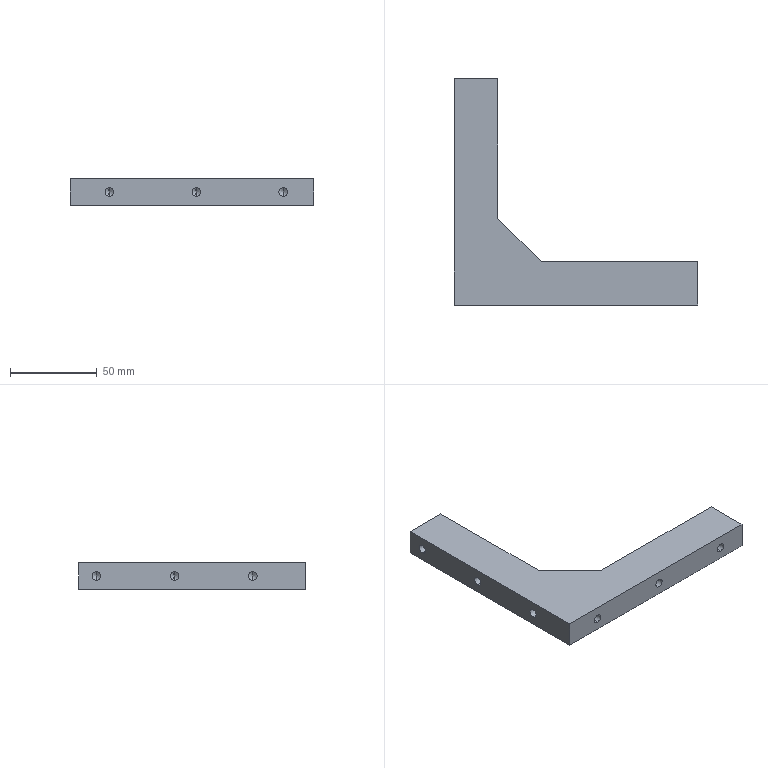Part | SolidWorks | features 3DProfileFeature 1, Extrusion 1, HoleWzd 1 | 1 solid | 33 faces | box 140 x 130 x 15 mm | volume 95031 mm3 | cylinder 12 | cone 12 | plane 9 | commonest cylinder face diameters 5 x12
STEP:
#1=CARTESIAN_POINT('',(122.5,12.5,2.5));
#2=VERTEX_POINT('',#1);
#3=CARTESIAN_POINT('',(122.5,12.5,-2.5));
#4=VERTEX_POINT('',#3);
#5=CARTESIAN_POINT('',(122.5,12.5,0.));
#6=DIRECTION('',(0.,-1.,0.));
#7=DIRECTION('',(0.,0.,-1.));
#8=AXIS2_PLACEMENT_3D('',#5,#6,#7);
#9=CIRCLE('',#8,2.5);
#10=EDGE_CURVE('',#2,#4,#9,.T.);
#11=ORIENTED_EDGE('',*,*,#10,.F.);
#12=CARTESIAN_POINT('',(122.5,0.,2.5));
#13=VERTEX_POINT('',#12);
#14=CARTESIAN_POINT('',(122.5,0.,2.5));
#15=DIRECTION('',(0.,-1.,0.));
#16=VECTOR('',#15,1000.);
#17=LINE('',#14,#16);
#18=EDGE_CURVE('',#2,#13,#17,.T.);
#19=ORIENTED_EDGE('',*,*,#18,.T.);
#20=CARTESIAN_POINT('',(122.5,0.,-2.5));
#21=VERTEX_POINT('',#20);
#22=CARTESIAN_POINT('',(122.5,0.,0.));
#23=DIRECTION('',(0.,-1.,0.));
#24=DIRECTION('',(0.,0.,-1.));
#25=AXIS2_PLACEMENT_3D('',#22,#23,#24);
#26=CIRCLE('',#25,2.5);
#27=EDGE_CURVE('',#13,#21,#26,.T.);
#28=ORIENTED_EDGE('',*,*,#27,.T.);
#29=CARTESIAN_POINT('',(122.5,0.,-2.5));
#30=DIRECTION('',(0.,-1.,0.));
#31=VECTOR('',#30,1000.);
#32=LINE('',#29,#31);
#33=EDGE_CURVE('',#4,#21,#32,.T.);
#34=ORIENTED_EDGE('',*,*,#33,.F.);
#35=EDGE_LOOP('',(#11,#19,#28,#34));
#36=FACE_OUTER_BOUND('',#35,.T.);
#37=CARTESIAN_POINT('',(122.5,0.,0.));
#38=DIRECTION('',(0.,-1.,0.));
#39=DIRECTION('',(0.,0.,-1.));
#40=AXIS2_PLACEMENT_3D('',#37,#38,#39);
#41=CYLINDRICAL_SURFACE('',#40,2.5);
#42=ADVANCED_FACE('',(#36),#41,.F.);
#43=CARTESIAN_POINT('',(122.5,14.002,0.));
#44=VERTEX_POINT('',#43);
#45=CARTESIAN_POINT('',(122.5,12.5,-2.5));
#46=DIRECTION('',(0.,-0.515,-0.8572));
#47=VECTOR('',#46,1000.);
#48=LINE('',#45,#47);
#49=EDGE_CURVE('',#44,#4,#48,.T.);
#50=ORIENTED_EDGE('',*,*,#49,.F.);
#51=CARTESIAN_POINT('',(122.5,12.5,2.5));
#52=DIRECTION('',(0.,-0.515,0.8572));
#53=VECTOR('',#52,1000.);
#54=LINE('',#51,#53);
#55=EDGE_CURVE('',#44,#2,#54,.T.);
#56=ORIENTED_EDGE('',*,*,#55,.T.);
#57=ORIENTED_EDGE('',*,*,#10,.T.);
#58=EDGE_LOOP('',(#50,#56,#57));
#59=FACE_OUTER_BOUND('',#58,.T.);
#60=CARTESIAN_POINT('',(122.5,12.5,0.));
#61=DIRECTION('',(0.,-1.,0.));
#62=DIRECTION('',(0.,0.,-1.));
#63=AXIS2_PLACEMENT_3D('',#60,#61,#62);
#64=CONICAL_SURFACE('',#63,2.5,1.03);
#65=ADVANCED_FACE('',(#59),#64,.F.);
#66=CARTESIAN_POINT('',(72.5,12.5,2.5));
#67=VERTEX_POINT('',#66);
#68=CARTESIAN_POINT('',(72.5,12.5,-2.5));
#69=VERTEX_POINT('',#68);
#70=CARTESIAN_POINT('',(72.5,12.5,0.));
#71=DIRECTION('',(0.,-1.,0.));
#72=DIRECTION('',(0.,0.,-1.));
#73=AXIS2_PLACEMENT_3D('',#70,#71,#72);
#74=CIRCLE('',#73,2.5);
#75=EDGE_CURVE('',#67,#69,#74,.T.);
#76=ORIENTED_EDGE('',*,*,#75,.F.);
#77=CARTESIAN_POINT('',(72.5,0.,2.5));
#78=VERTEX_POINT('',#77);
#79=CARTESIAN_POINT('',(72.5,0.,2.5));
#80=DIRECTION('',(0.,-1.,0.));
#81=VECTOR('',#80,1000.);
#82=LINE('',#79,#81);
#83=EDGE_CURVE('',#67,#78,#82,.T.);
#84=ORIENTED_EDGE('',*,*,#83,.T.);
#85=CARTESIAN_POINT('',(72.5,0.,-2.5));
#86=VERTEX_POINT('',#85);
#87=CARTESIAN_POINT('',(72.5,0.,0.));
#88=DIRECTION('',(0.,-1.,0.));
#89=DIRECTION('',(0.,0.,-1.));
#90=AXIS2_PLACEMENT_3D('',#87,#88,#89);
#91=CIRCLE('',#90,2.5);
#92=EDGE_CURVE('',#78,#86,#91,.T.);
#93=ORIENTED_EDGE('',*,*,#92,.T.);
#94=CARTESIAN_POINT('',(72.5,0.,-2.5));
#95=DIRECTION('',(0.,-1.,0.));
#96=VECTOR('',#95,1000.);
#97=LINE('',#94,#96);
#98=EDGE_CURVE('',#69,#86,#97,.T.);
#99=ORIENTED_EDGE('',*,*,#98,.F.);
#100=EDGE_LOOP('',(#76,#84,#93,#99));
#101=FACE_OUTER_BOUND('',#100,.T.);
#102=CARTESIAN_POINT('',(72.5,0.,0.));
#103=DIRECTION('',(0.,-1.,0.));
#104=DIRECTION('',(0.,0.,-1.));
#105=AXIS2_PLACEMENT_3D('',#102,#103,#104);
#106=CYLINDRICAL_SURFACE('',#105,2.5);
#107=ADVANCED_FACE('',(#101),#106,.F.);
#108=CARTESIAN_POINT('',(72.5,14.002,0.));
#109=VERTEX_POINT('',#108);
#110=CARTESIAN_POINT('',(72.5,12.5,-2.5));
#111=DIRECTION('',(0.,-0.515,-0.8572));
#112=VECTOR('',#111,1000.);
#113=LINE('',#110,#112);
#114=EDGE_CURVE('',#109,#69,#113,.T.);
#115=ORIENTED_EDGE('',*,*,#114,.F.);
#116=CARTESIAN_POINT('',(72.5,12.5,2.5));
#117=DIRECTION('',(0.,-0.515,0.8572));
#118=VECTOR('',#117,1000.);
#119=LINE('',#116,#118);
#120=EDGE_CURVE('',#109,#67,#119,.T.);
#121=ORIENTED_EDGE('',*,*,#120,.T.);
#122=ORIENTED_EDGE('',*,*,#75,.T.);
#123=EDGE_LOOP('',(#115,#121,#122));
#124=FACE_OUTER_BOUND('',#123,.T.);
#125=CARTESIAN_POINT('',(72.5,12.5,0.));
#126=DIRECTION('',(0.,-1.,0.));
#127=DIRECTION('',(0.,0.,-1.));
#128=AXIS2_PLACEMENT_3D('',#125,#126,#127);
#129=CONICAL_SURFACE('',#128,2.5,1.03);
#130=ADVANCED_FACE('',(#124),#129,.F.);
#131=CARTESIAN_POINT('',(22.5,12.5,2.5));
#132=VERTEX_POINT('',#131);
#133=CARTESIAN_POINT('',(22.5,12.5,-2.5));
#134=VERTEX_POINT('',#133);
#135=CARTESIAN_POINT('',(22.5,12.5,0.));
#136=DIRECTION('',(0.,-1.,0.));
#137=DIRECTION('',(0.,0.,-1.));
#138=AXIS2_PLACEMENT_3D('',#135,#136,#137);
#139=CIRCLE('',#138,2.5);
#140=EDGE_CURVE('',#132,#134,#139,.T.);
#141=ORIENTED_EDGE('',*,*,#140,.F.);
#142=CARTESIAN_POINT('',(22.5,0.,2.5));
#143=VERTEX_POINT('',#142);
#144=CARTESIAN_POINT('',(22.5,0.,2.5));
#145=DIRECTION('',(0.,-1.,0.));
#146=VECTOR('',#145,1000.);
#147=LINE('',#144,#146);
#148=EDGE_CURVE('',#132,#143,#147,.T.);
#149=ORIENTED_EDGE('',*,*,#148,.T.);
#150=CARTESIAN_POINT('',(22.5,0.,-2.5));
#151=VERTEX_POINT('',#150);
#152=CARTESIAN_POINT('',(22.5,0.,0.));
#153=DIRECTION('',(0.,-1.,0.));
#154=DIRECTION('',(0.,0.,-1.));
#155=AXIS2_PLACEMENT_3D('',#152,#153,#154);
#156=CIRCLE('',#155,2.5);
#157=EDGE_CURVE('',#143,#151,#156,.T.);
#158=ORIENTED_EDGE('',*,*,#157,.T.);
#159=CARTESIAN_POINT('',(22.5,0.,-2.5));
#160=DIRECTION('',(0.,-1.,0.));
#161=VECTOR('',#160,1000.);
#162=LINE('',#159,#161);
#163=EDGE_CURVE('',#134,#151,#162,.T.);
#164=ORIENTED_EDGE('',*,*,#163,.F.);
#165=EDGE_LOOP('',(#141,#149,#158,#164));
#166=FACE_OUTER_BOUND('',#165,.T.);
#167=CARTESIAN_POINT('',(22.5,0.,0.));
#168=DIRECTION('',(0.,-1.,0.));
#169=DIRECTION('',(0.,0.,-1.));
#170=AXIS2_PLACEMENT_3D('',#167,#168,#169);
#171=CYLINDRICAL_SURFACE('',#170,2.5);
#172=ADVANCED_FACE('',(#166),#171,.F.);
#173=CARTESIAN_POINT('',(22.5,14.002,0.));
#174=VERTEX_POINT('',#173);
#175=CARTESIAN_POINT('',(22.5,12.5,-2.5));
#176=DIRECTION('',(0.,-0.515,-0.8572));
#177=VECTOR('',#176,1000.);
#178=LINE('',#175,#177);
#179=EDGE_CURVE('',#174,#134,#178,.T.);
#180=ORIENTED_EDGE('',*,*,#179,.F.);
#181=CARTESIAN_POINT('',(22.5,12.5,2.5));
#182=DIRECTION('',(0.,-0.515,0.8572));
#183=VECTOR('',#182,1000.);
#184=LINE('',#181,#183);
#185=EDGE_CURVE('',#174,#132,#184,.T.);
#186=ORIENTED_EDGE('',*,*,#185,.T.);
#187=ORIENTED_EDGE('',*,*,#140,.T.);
#188=EDGE_LOOP('',(#180,#186,#187));
#189=FACE_OUTER_BOUND('',#188,.T.);
#190=CARTESIAN_POINT('',(22.5,12.5,0.));
#191=DIRECTION('',(0.,-1.,0.));
#192=DIRECTION('',(0.,0.,-1.));
#193=AXIS2_PLACEMENT_3D('',#190,#191,#192);
#194=CONICAL_SURFACE('',#193,2.5,1.03);
#195=ADVANCED_FACE('',(#189),#194,.F.);
#196=CARTESIAN_POINT('',(12.5,30.,-2.5));
#197=VERTEX_POINT('',#196);
#198=CARTESIAN_POINT('',(12.5,30.,2.5));
#199=VERTEX_POINT('',#198);
#200=CARTESIAN_POINT('',(12.5,30.,0.));
#201=DIRECTION('',(-1.,0.,0.));
#202=DIRECTION('',(0.,0.,1.));
#203=AXIS2_PLACEMENT_3D('',#200,#201,#202);
#204=CIRCLE('',#203,2.5);
#205=EDGE_CURVE('',#197,#199,#204,.T.);
#206=ORIENTED_EDGE('',*,*,#205,.F.);
#207=CARTESIAN_POINT('',(0.,30.,-2.5));
#208=VERTEX_POINT('',#207);
#209=CARTESIAN_POINT('',(0.,30.,-2.5));
#210=DIRECTION('',(-1.,0.,0.));
#211=VECTOR('',#210,1000.);
#212=LINE('',#209,#211);
#213=EDGE_CURVE('',#197,#208,#212,.T.);
#214=ORIENTED_EDGE('',*,*,#213,.T.);
#215=CARTESIAN_POINT('',(0.,30.,2.5));
#216=VERTEX_POINT('',#215);
#217=CARTESIAN_POINT('',(0.,30.,0.));
#218=DIRECTION('',(-1.,0.,0.));
#219=DIRECTION('',(0.,0.,1.));
#220=AXIS2_PLACEMENT_3D('',#217,#218,#219);
#221=CIRCLE('',#220,2.5);
#222=EDGE_CURVE('',#208,#216,#221,.T.);
#223=ORIENTED_EDGE('',*,*,#222,.T.);
#224=CARTESIAN_POINT('',(0.,30.,2.5));
#225=DIRECTION('',(-1.,0.,0.));
#226=VECTOR('',#225,1000.);
#227=LINE('',#224,#226);
#228=EDGE_CURVE('',#199,#216,#227,.T.);
#229=ORIENTED_EDGE('',*,*,#228,.F.);
#230=EDGE_LOOP('',(#206,#214,#223,#229));
#231=FACE_OUTER_BOUND('',#230,.T.);
#232=CARTESIAN_POINT('',(0.,30.,0.));
#233=DIRECTION('',(-1.,0.,0.));
#234=DIRECTION('',(0.,0.,1.));
#235=AXIS2_PLACEMENT_3D('',#232,#233,#234);
#236=CYLINDRICAL_SURFACE('',#235,2.5);
#237=ADVANCED_FACE('',(#231),#236,.F.);
#238=CARTESIAN_POINT('',(14.002,30.,0.));
#239=VERTEX_POINT('',#238);
#240=CARTESIAN_POINT('',(12.5,30.,2.5));
#241=DIRECTION('',(-0.515,0.,0.8572));
#242=VECTOR('',#241,1000.);
#243=LINE('',#240,#242);
#244=EDGE_CURVE('',#239,#199,#243,.T.);
#245=ORIENTED_EDGE('',*,*,#244,.F.);
#246=CARTESIAN_POINT('',(12.5,30.,-2.5));
#247=DIRECTION('',(-0.515,0.,-0.8572));
#248=VECTOR('',#247,1000.);
#249=LINE('',#246,#248);
#250=EDGE_CURVE('',#239,#197,#249,.T.);
#251=ORIENTED_EDGE('',*,*,#250,.T.);
#252=ORIENTED_EDGE('',*,*,#205,.T.);
#253=EDGE_LOOP('',(#245,#251,#252));
#254=FACE_OUTER_BOUND('',#253,.T.);
#255=CARTESIAN_POINT('',(12.5,30.,0.));
#256=DIRECTION('',(-1.,0.,0.));
#257=DIRECTION('',(0.,0.,1.));
#258=AXIS2_PLACEMENT_3D('',#255,#256,#257);
#259=CONICAL_SURFACE('',#258,2.5,1.03);
#260=ADVANCED_FACE('',(#254),#259,.F.);
#261=CARTESIAN_POINT('',(12.5,75.,-2.5));
#262=VERTEX_POINT('',#261);
#263=CARTESIAN_POINT('',(12.5,75.,2.5));
#264=VERTEX_POINT('',#263);
#265=CARTESIAN_POINT('',(12.5,75.,0.));
#266=DIRECTION('',(-1.,0.,0.));
#267=DIRECTION('',(0.,0.,1.));
#268=AXIS2_PLACEMENT_3D('',#265,#266,#267);
#269=CIRCLE('',#268,2.5);
#270=EDGE_CURVE('',#262,#264,#269,.T.);
#271=ORIENTED_EDGE('',*,*,#270,.F.);
#272=CARTESIAN_POINT('',(0.,75.,-2.5));
#273=VERTEX_POINT('',#272);
#274=CARTESIAN_POINT('',(0.,75.,-2.5));
#275=DIRECTION('',(-1.,0.,0.));
#276=VECTOR('',#275,1000.);
#277=LINE('',#274,#276);
#278=EDGE_CURVE('',#262,#273,#277,.T.);
#279=ORIENTED_EDGE('',*,*,#278,.T.);
#280=CARTESIAN_POINT('',(0.,75.,2.5));
#281=VERTEX_POINT('',#280);
#282=CARTESIAN_POINT('',(0.,75.,0.));
#283=DIRECTION('',(-1.,0.,0.));
#284=DIRECTION('',(0.,0.,1.));
#285=AXIS2_PLACEMENT_3D('',#282,#283,#284);
#286=CIRCLE('',#285,2.5);
#287=EDGE_CURVE('',#273,#281,#286,.T.);
#288=ORIENTED_EDGE('',*,*,#287,.T.);
#289=CARTESIAN_POINT('',(0.,75.,2.5));
#290=DIRECTION('',(-1.,0.,0.));
#291=VECTOR('',#290,1000.);
#292=LINE('',#289,#291);
#293=EDGE_CURVE('',#264,#281,#292,.T.);
#294=ORIENTED_EDGE('',*,*,#293,.F.);
#295=EDGE_LOOP('',(#271,#279,#288,#294));
#296=FACE_OUTER_BOUND('',#295,.T.);
#297=CARTESIAN_POINT('',(0.,75.,0.));
#298=DIRECTION('',(-1.,0.,0.));
#299=DIRECTION('',(0.,0.,1.));
#300=AXIS2_PLACEMENT_3D('',#297,#298,#299);
#301=CYLINDRICAL_SURFACE('',#300,2.5);
#302=ADVANCED_FACE('',(#296),#301,.F.);
#303=CARTESIAN_POINT('',(14.002,75.,0.));
#304=VERTEX_POINT('',#303);
#305=CARTESIAN_POINT('',(12.5,75.,2.5));
#306=DIRECTION('',(-0.515,0.,0.8572));
#307=VECTOR('',#306,1000.);
#308=LINE('',#305,#307);
#309=EDGE_CURVE('',#304,#264,#308,.T.);
#310=ORIENTED_EDGE('',*,*,#309,.F.);
#311=CARTESIAN_POINT('',(12.5,75.,-2.5));
#312=DIRECTION('',(-0.515,0.,-0.8572));
#313=VECTOR('',#312,1000.);
#314=LINE('',#311,#313);
#315=EDGE_CURVE('',#304,#262,#314,.T.);
#316=ORIENTED_EDGE('',*,*,#315,.T.);
#317=ORIENTED_EDGE('',*,*,#270,.T.);
#318=EDGE_LOOP('',(#310,#316,#317));
#319=FACE_OUTER_BOUND('',#318,.T.);
#320=CARTESIAN_POINT('',(12.5,75.,0.));
#321=DIRECTION('',(-1.,0.,0.));
#322=DIRECTION('',(0.,0.,1.));
#323=AXIS2_PLACEMENT_3D('',#320,#321,#322);
#324=CONICAL_SURFACE('',#323,2.5,1.03);
#325=ADVANCED_FACE('',(#319),#324,.F.);
#326=CARTESIAN_POINT('',(12.5,120.,-2.5));
#327=VERTEX_POINT('',#326);
#328=CARTESIAN_POINT('',(12.5,120.,2.5));
#329=VERTEX_POINT('',#328);
#330=CARTESIAN_POINT('',(12.5,120.,0.));
#331=DIRECTION('',(-1.,0.,0.));
#332=DIRECTION('',(0.,0.,1.));
#333=AXIS2_PLACEMENT_3D('',#330,#331,#332);
#334=CIRCLE('',#333,2.5);
#335=EDGE_CURVE('',#327,#329,#334,.T.);
#336=ORIENTED_EDGE('',*,*,#335,.F.);
#337=CARTESIAN_POINT('',(0.,120.,-2.5));
#338=VERTEX_POINT('',#337);
#339=CARTESIAN_POINT('',(0.,120.,-2.5));
#340=DIRECTION('',(-1.,0.,0.));
#341=VECTOR('',#340,1000.);
#342=LINE('',#339,#341);
#343=EDGE_CURVE('',#327,#338,#342,.T.);
#344=ORIENTED_EDGE('',*,*,#343,.T.);
#345=CARTESIAN_POINT('',(0.,120.,2.5));
#346=VERTEX_POINT('',#345);
#347=CARTESIAN_POINT('',(0.,120.,0.));
#348=DIRECTION('',(-1.,0.,0.));
#349=DIRECTION('',(0.,0.,1.));
#350=AXIS2_PLACEMENT_3D('',#347,#348,#349);
#351=CIRCLE('',#350,2.5);
#352=EDGE_CURVE('',#338,#346,#351,.T.);
#353=ORIENTED_EDGE('',*,*,#352,.T.);
#354=CARTESIAN_POINT('',(0.,120.,2.5));
#355=DIRECTION('',(-1.,0.,0.));
#356=VECTOR('',#355,1000.);
#357=LINE('',#354,#356);
#358=EDGE_CURVE('',#329,#346,#357,.T.);
#359=ORIENTED_EDGE('',*,*,#358,.F.);
#360=EDGE_LOOP('',(#336,#344,#353,#359));
#361=FACE_OUTER_BOUND('',#360,.T.);
#362=CARTESIAN_POINT('',(0.,120.,0.));
#363=DIRECTION('',(-1.,0.,0.));
#364=DIRECTION('',(0.,0.,1.));
#365=AXIS2_PLACEMENT_3D('',#362,#363,#364);
#366=CYLINDRICAL_SURFACE('',#365,2.5);
#367=ADVANCED_FACE('',(#361),#366,.F.);
#368=CARTESIAN_POINT('',(14.002,120.,0.));
#369=VERTEX_POINT('',#368);
#370=CARTESIAN_POINT('',(12.5,120.,2.5));
#371=DIRECTION('',(-0.515,0.,0.8572));
#372=VECTOR('',#371,1000.);
#373=LINE('',#370,#372);
#374=EDGE_CURVE('',#369,#329,#373,.T.);
#375=ORIENTED_EDGE('',*,*,#374,.F.);
#376=CARTESIAN_POINT('',(12.5,120.,-2.5));
#377=DIRECTION('',(-0.515,0.,-0.8572));
#378=VECTOR('',#377,1000.);
#379=LINE('',#376,#378);
#380=EDGE_CURVE('',#369,#327,#379,.T.);
#381=ORIENTED_EDGE('',*,*,#380,.T.);
#382=ORIENTED_EDGE('',*,*,#335,.T.);
#383=EDGE_LOOP('',(#375,#381,#382));
#384=FACE_OUTER_BOUND('',#383,.T.);
#385=CARTESIAN_POINT('',(12.5,120.,0.));
#386=DIRECTION('',(-1.,0.,0.));
#387=DIRECTION('',(0.,0.,1.));
#388=AXIS2_PLACEMENT_3D('',#385,#386,#387);
#389=CONICAL_SURFACE('',#388,2.5,1.03);
#390=ADVANCED_FACE('',(#384),#389,.F.);
#391=CARTESIAN_POINT('',(25.,130.,-7.5));
#392=VERTEX_POINT('',#391);
#393=CARTESIAN_POINT('',(0.,130.,-7.5));
#394=VERTEX_POINT('',#393);
#395=CARTESIAN_POINT('',(25.,130.,-7.5));
#396=DIRECTION('',(-1.,0.,0.));
#397=VECTOR('',#396,1000.);
#398=LINE('',#395,#397);
#399=EDGE_CURVE('',#392,#394,#398,.T.);
#400=ORIENTED_EDGE('',*,*,#399,.T.);
#401=CARTESIAN_POINT('',(0.,130.,7.5));
#402=VERTEX_POINT('',#401);
#403=CARTESIAN_POINT('',(0.,130.,7.5));
#404=DIRECTION('',(0.,0.,-1.));
#405=VECTOR('',#404,1000.);
#406=LINE('',#403,#405);
#407=EDGE_CURVE('',#402,#394,#406,.T.);
#408=ORIENTED_EDGE('',*,*,#407,.F.);
#409=CARTESIAN_POINT('',(25.,130.,7.5));
#410=VERTEX_POINT('',#409);
#411=CARTESIAN_POINT('',(25.,130.,7.5));
#412=DIRECTION('',(-1.,0.,0.));
#413=VECTOR('',#412,1000.);
#414=LINE('',#411,#413);
#415=EDGE_CURVE('',#410,#402,#414,.T.);
#416=ORIENTED_EDGE('',*,*,#415,.F.);
#417=CARTESIAN_POINT('',(25.,130.,7.5));
#418=DIRECTION('',(0.,0.,-1.));
#419=VECTOR('',#418,1000.);
#420=LINE('',#417,#419);
#421=EDGE_CURVE('',#410,#392,#420,.T.);
#422=ORIENTED_EDGE('',*,*,#421,.T.);
#423=EDGE_LOOP('',(#400,#408,#416,#422));
#424=FACE_OUTER_BOUND('',#423,.T.);
#425=CARTESIAN_POINT('',(25.,130.,7.5));
#426=DIRECTION('',(0.,-1.,0.));
#427=DIRECTION('',(0.,0.,-1.));
#428=AXIS2_PLACEMENT_3D('',#425,#426,#427);
#429=PLANE('',#428);
#430=ADVANCED_FACE('',(#424),#429,.F.);
#431=CARTESIAN_POINT('',(0.,30.,0.));
#432=DIRECTION('',(-1.,0.,0.));
#433=DIRECTION('',(0.,0.,1.));
#434=AXIS2_PLACEMENT_3D('',#431,#432,#433);
#435=CIRCLE('',#434,2.5);
#436=EDGE_CURVE('',#216,#208,#435,.T.);
#437=ORIENTED_EDGE('',*,*,#436,.F.);
#438=ORIENTED_EDGE('',*,*,#222,.F.);
#439=EDGE_LOOP('',(#437,#438));
#440=FACE_BOUND('',#439,.T.);
#441=CARTESIAN_POINT('',(0.,75.,0.));
#442=DIRECTION('',(-1.,0.,0.));
#443=DIRECTION('',(0.,0.,1.));
#444=AXIS2_PLACEMENT_3D('',#441,#442,#443);
#445=CIRCLE('',#444,2.5);
#446=EDGE_CURVE('',#281,#273,#445,.T.);
#447=ORIENTED_EDGE('',*,*,#446,.F.);
#448=ORIENTED_EDGE('',*,*,#287,.F.);
#449=EDGE_LOOP('',(#447,#448));
#450=FACE_BOUND('',#449,.T.);
#451=CARTESIAN_POINT('',(0.,120.,0.));
#452=DIRECTION('',(-1.,0.,0.));
#453=DIRECTION('',(0.,0.,1.));
#454=AXIS2_PLACEMENT_3D('',#451,#452,#453);
#455=CIRCLE('',#454,2.5);
#456=EDGE_CURVE('',#346,#338,#455,.T.);
#457=ORIENTED_EDGE('',*,*,#456,.F.);
#458=ORIENTED_EDGE('',*,*,#352,.F.);
#459=EDGE_LOOP('',(#457,#458));
#460=FACE_BOUND('',#459,.T.);
#461=CARTESIAN_POINT('',(0.,0.,-7.5));
#462=VERTEX_POINT('',#461);
#463=CARTESIAN_POINT('',(0.,130.,-7.5));
#464=DIRECTION('',(0.,-1.,0.));
#465=VECTOR('',#464,1000.);
#466=LINE('',#463,#465);
#467=EDGE_CURVE('',#394,#462,#466,.T.);
#468=ORIENTED_EDGE('',*,*,#467,.T.);
#469=CARTESIAN_POINT('',(0.,0.,7.5));
#470=VERTEX_POINT('',#469);
#471=CARTESIAN_POINT('',(0.,0.,7.5));
#472=DIRECTION('',(0.,0.,-1.));
#473=VECTOR('',#472,1000.);
#474=LINE('',#471,#473);
#475=EDGE_CURVE('',#470,#462,#474,.T.);
#476=ORIENTED_EDGE('',*,*,#475,.F.);
#477=CARTESIAN_POINT('',(0.,130.,7.5));
#478=DIRECTION('',(0.,-1.,0.));
#479=VECTOR('',#478,1000.);
#480=LINE('',#477,#479);
#481=EDGE_CURVE('',#402,#470,#480,.T.);
#482=ORIENTED_EDGE('',*,*,#481,.F.);
#483=ORIENTED_EDGE('',*,*,#407,.T.);
#484=EDGE_LOOP('',(#468,#476,#482,#483));
#485=FACE_OUTER_BOUND('',#484,.T.);
#486=CARTESIAN_POINT('',(0.,130.,7.5));
#487=DIRECTION('',(1.,0.,0.));
#488=DIRECTION('',(0.,1.,0.));
#489=AXIS2_PLACEMENT_3D('',#486,#487,#488);
#490=PLANE('',#489);
#491=ADVANCED_FACE('',(#440,#450,#460,#485),#490,.F.);
#492=CARTESIAN_POINT('',(122.5,0.,0.));
#493=DIRECTION('',(0.,-1.,0.));
#494=DIRECTION('',(0.,0.,-1.));
#495=AXIS2_PLACEMENT_3D('',#492,#493,#494);
#496=CIRCLE('',#495,2.5);
#497=EDGE_CURVE('',#21,#13,#496,.T.);
#498=ORIENTED_EDGE('',*,*,#497,.F.);
#499=ORIENTED_EDGE('',*,*,#27,.F.);
#500=EDGE_LOOP('',(#498,#499));
#501=FACE_BOUND('',#500,.T.);
#502=CARTESIAN_POINT('',(72.5,0.,0.));
#503=DIRECTION('',(0.,-1.,0.));
#504=DIRECTION('',(0.,0.,-1.));
#505=AXIS2_PLACEMENT_3D('',#502,#503,#504);
#506=CIRCLE('',#505,2.5);
#507=EDGE_CURVE('',#86,#78,#506,.T.);
#508=ORIENTED_EDGE('',*,*,#507,.F.);
#509=ORIENTED_EDGE('',*,*,#92,.F.);
#510=EDGE_LOOP('',(#508,#509));
#511=FACE_BOUND('',#510,.T.);
#512=CARTESIAN_POINT('',(22.5,0.,0.));
#513=DIRECTION('',(0.,-1.,0.));
#514=DIRECTION('',(0.,0.,-1.));
#515=AXIS2_PLACEMENT_3D('',#512,#513,#514);
#516=CIRCLE('',#515,2.5);
#517=EDGE_CURVE('',#151,#143,#516,.T.);
#518=ORIENTED_EDGE('',*,*,#517,.F.);
#519=ORIENTED_EDGE('',*,*,#157,.F.);
#520=EDGE_LOOP('',(#518,#519));
#521=FACE_BOUND('',#520,.T.);
#522=CARTESIAN_POINT('',(140.,0.,-7.5));
#523=VERTEX_POINT('',#522);
#524=CARTESIAN_POINT('',(0.,0.,-7.5));
#525=DIRECTION('',(1.,0.,0.));
#526=VECTOR('',#525,1000.);
#527=LINE('',#524,#526);
#528=EDGE_CURVE('',#462,#523,#527,.T.);
#529=ORIENTED_EDGE('',*,*,#528,.T.);
#530=CARTESIAN_POINT('',(140.,0.,7.5));
#531=VERTEX_POINT('',#530);
#532=CARTESIAN_POINT('',(140.,0.,7.5));
#533=DIRECTION('',(0.,0.,-1.));
#534=VECTOR('',#533,1000.);
#535=LINE('',#532,#534);
#536=EDGE_CURVE('',#531,#523,#535,.T.);
#537=ORIENTED_EDGE('',*,*,#536,.F.);
#538=CARTESIAN_POINT('',(0.,0.,7.5));
#539=DIRECTION('',(1.,0.,0.));
#540=VECTOR('',#539,1000.);
#541=LINE('',#538,#540);
#542=EDGE_CURVE('',#470,#531,#541,.T.);
#543=ORIENTED_EDGE('',*,*,#542,.F.);
#544=ORIENTED_EDGE('',*,*,#475,.T.);
#545=EDGE_LOOP('',(#529,#537,#543,#544));
#546=FACE_OUTER_BOUND('',#545,.T.);
#547=CARTESIAN_POINT('',(0.,0.,7.5));
#548=DIRECTION('',(0.,1.,0.));
#549=DIRECTION('',(0.,0.,1.));
#550=AXIS2_PLACEMENT_3D('',#547,#548,#549);
#551=PLANE('',#550);
#552=ADVANCED_FACE('',(#501,#511,#521,#546),#551,.F.);
#553=CARTESIAN_POINT('',(140.,25.,-7.5));
#554=VERTEX_POINT('',#553);
#555=CARTESIAN_POINT('',(140.,0.,-7.5));
#556=DIRECTION('',(0.,1.,0.));
#557=VECTOR('',#556,1000.);
#558=LINE('',#555,#557);
#559=EDGE_CURVE('',#523,#554,#558,.T.);
#560=ORIENTED_EDGE('',*,*,#559,.T.);
#561=CARTESIAN_POINT('',(140.,25.,7.5));
#562=VERTEX_POINT('',#561);
#563=CARTESIAN_POINT('',(140.,25.,7.5));
#564=DIRECTION('',(0.,0.,-1.));
#565=VECTOR('',#564,1000.);
#566=LINE('',#563,#565);
#567=EDGE_CURVE('',#562,#554,#566,.T.);
#568=ORIENTED_EDGE('',*,*,#567,.F.);
#569=CARTESIAN_POINT('',(140.,0.,7.5));
#570=DIRECTION('',(0.,1.,0.));
#571=VECTOR('',#570,1000.);
#572=LINE('',#569,#571);
#573=EDGE_CURVE('',#531,#562,#572,.T.);
#574=ORIENTED_EDGE('',*,*,#573,.F.);
#575=ORIENTED_EDGE('',*,*,#536,.T.);
#576=EDGE_LOOP('',(#560,#568,#574,#575));
#577=FACE_OUTER_BOUND('',#576,.T.);
#578=CARTESIAN_POINT('',(140.,0.,7.5));
#579=DIRECTION('',(-1.,0.,0.));
#580=DIRECTION('',(0.,0.,1.));
#581=AXIS2_PLACEMENT_3D('',#578,#579,#580);
#582=PLANE('',#581);
#583=ADVANCED_FACE('',(#577),#582,.F.);
#584=CARTESIAN_POINT('',(50.,25.,-7.5));
#585=VERTEX_POINT('',#584);
#586=CARTESIAN_POINT('',(140.,25.,-7.5));
#587=DIRECTION('',(-1.,0.,0.));
#588=VECTOR('',#587,1000.);
#589=LINE('',#586,#588);
#590=EDGE_CURVE('',#554,#585,#589,.T.);
#591=ORIENTED_EDGE('',*,*,#590,.T.);
#592=CARTESIAN_POINT('',(50.,25.,7.5));
#593=VERTEX_POINT('',#592);
#594=CARTESIAN_POINT('',(50.,25.,7.5));
#595=DIRECTION('',(0.,0.,-1.));
#596=VECTOR('',#595,1000.);
#597=LINE('',#594,#596);
#598=EDGE_CURVE('',#593,#585,#597,.T.);
#599=ORIENTED_EDGE('',*,*,#598,.F.);
#600=CARTESIAN_POINT('',(140.,25.,7.5));
#601=DIRECTION('',(-1.,0.,0.));
#602=VECTOR('',#601,1000.);
#603=LINE('',#600,#602);
#604=EDGE_CURVE('',#562,#593,#603,.T.);
#605=ORIENTED_EDGE('',*,*,#604,.F.);
#606=ORIENTED_EDGE('',*,*,#567,.T.);
#607=EDGE_LOOP('',(#591,#599,#605,#606));
#608=FACE_OUTER_BOUND('',#607,.T.);
#609=CARTESIAN_POINT('',(140.,25.,7.5));
#610=DIRECTION('',(0.,-1.,0.));
#611=DIRECTION('',(1.,0.,0.));
#612=AXIS2_PLACEMENT_3D('',#609,#610,#611);
#613=PLANE('',#612);
#614=ADVANCED_FACE('',(#608),#613,.F.);
#615=CARTESIAN_POINT('',(25.,50.,-7.5));
#616=VERTEX_POINT('',#615);
#617=CARTESIAN_POINT('',(50.,25.,-7.5));
#618=DIRECTION('',(-0.7071,0.7071,0.));
#619=VECTOR('',#618,1000.);
#620=LINE('',#617,#619);
#621=EDGE_CURVE('',#585,#616,#620,.T.);
#622=ORIENTED_EDGE('',*,*,#621,.T.);
#623=CARTESIAN_POINT('',(25.,50.,7.5));
#624=VERTEX_POINT('',#623);
#625=CARTESIAN_POINT('',(25.,50.,7.5));
#626=DIRECTION('',(0.,0.,-1.));
#627=VECTOR('',#626,1000.);
#628=LINE('',#625,#627);
#629=EDGE_CURVE('',#624,#616,#628,.T.);
#630=ORIENTED_EDGE('',*,*,#629,.F.);
#631=CARTESIAN_POINT('',(50.,25.,7.5));
#632=DIRECTION('',(-0.7071,0.7071,0.));
#633=VECTOR('',#632,1000.);
#634=LINE('',#631,#633);
#635=EDGE_CURVE('',#593,#624,#634,.T.);
#636=ORIENTED_EDGE('',*,*,#635,.F.);
#637=ORIENTED_EDGE('',*,*,#598,.T.);
#638=EDGE_LOOP('',(#622,#630,#636,#637));
#639=FACE_OUTER_BOUND('',#638,.T.);
#640=CARTESIAN_POINT('',(50.,25.,7.5));
#641=DIRECTION('',(-0.7071,-0.7071,0.));
#642=DIRECTION('',(0.7071,-0.7071,0.));
#643=AXIS2_PLACEMENT_3D('',#640,#641,#642);
#644=PLANE('',#643);
#645=ADVANCED_FACE('',(#639),#644,.F.);
#646=CARTESIAN_POINT('',(25.,50.,-7.5));
#647=DIRECTION('',(0.,1.,0.));
#648=VECTOR('',#647,1000.);
#649=LINE('',#646,#648);
#650=EDGE_CURVE('',#616,#392,#649,.T.);
#651=ORIENTED_EDGE('',*,*,#650,.T.);
#652=ORIENTED_EDGE('',*,*,#421,.F.);
#653=CARTESIAN_POINT('',(25.,50.,7.5));
#654=DIRECTION('',(0.,1.,0.));
#655=VECTOR('',#654,1000.);
#656=LINE('',#653,#655);
#657=EDGE_CURVE('',#624,#410,#656,.T.);
#658=ORIENTED_EDGE('',*,*,#657,.F.);
#659=ORIENTED_EDGE('',*,*,#629,.T.);
#660=EDGE_LOOP('',(#651,#652,#658,#659));
#661=FACE_OUTER_BOUND('',#660,.T.);
#662=CARTESIAN_POINT('',(25.,50.,7.5));
#663=DIRECTION('',(-1.,0.,0.));
#664=DIRECTION('',(0.,0.,1.));
#665=AXIS2_PLACEMENT_3D('',#662,#663,#664);
#666=PLANE('',#665);
#667=ADVANCED_FACE('',(#661),#666,.F.);
#668=ORIENTED_EDGE('',*,*,#415,.T.);
#669=ORIENTED_EDGE('',*,*,#481,.T.);
#670=ORIENTED_EDGE('',*,*,#542,.T.);
#671=ORIENTED_EDGE('',*,*,#573,.T.);
#672=ORIENTED_EDGE('',*,*,#604,.T.);
#673=ORIENTED_EDGE('',*,*,#635,.T.);
#674=ORIENTED_EDGE('',*,*,#657,.T.);
#675=EDGE_LOOP('',(#668,#669,#670,#671,#672,#673,#674));
#676=FACE_OUTER_BOUND('',#675,.T.);
#677=CARTESIAN_POINT('',(0.,0.,7.5));
#678=DIRECTION('',(0.,0.,1.));
#679=DIRECTION('',(1.,0.,0.));
#680=AXIS2_PLACEMENT_3D('',#677,#678,#679);
#681=PLANE('',#680);
#682=ADVANCED_FACE('',(#676),#681,.T.);
#683=ORIENTED_EDGE('',*,*,#399,.F.);
#684=ORIENTED_EDGE('',*,*,#650,.F.);
#685=ORIENTED_EDGE('',*,*,#621,.F.);
#686=ORIENTED_EDGE('',*,*,#590,.F.);
#687=ORIENTED_EDGE('',*,*,#559,.F.);
#688=ORIENTED_EDGE('',*,*,#528,.F.);
#689=ORIENTED_EDGE('',*,*,#467,.F.);
#690=EDGE_LOOP('',(#683,#684,#685,#686,#687,#688,#689));
#691=FACE_OUTER_BOUND('',#690,.T.);
#692=CARTESIAN_POINT('',(0.,0.,-7.5));
#693=DIRECTION('',(0.,0.,1.));
#694=DIRECTION('',(1.,0.,0.));
#695=AXIS2_PLACEMENT_3D('',#692,#693,#694);
#696=PLANE('',#695);
#697=ADVANCED_FACE('',(#691),#696,.F.);
#698=ORIENTED_EDGE('',*,*,#380,.F.);
#699=ORIENTED_EDGE('',*,*,#374,.T.);
#700=CARTESIAN_POINT('',(12.5,120.,0.));
#701=DIRECTION('',(-1.,0.,0.));
#702=DIRECTION('',(0.,0.,1.));
#703=AXIS2_PLACEMENT_3D('',#700,#701,#702);
#704=CIRCLE('',#703,2.5);
#705=EDGE_CURVE('',#329,#327,#704,.T.);
#706=ORIENTED_EDGE('',*,*,#705,.T.);
#707=EDGE_LOOP('',(#698,#699,#706));
#708=FACE_OUTER_BOUND('',#707,.T.);
#709=CARTESIAN_POINT('',(12.5,120.,0.));
#710=DIRECTION('',(-1.,0.,0.));
#711=DIRECTION('',(0.,0.,1.));
#712=AXIS2_PLACEMENT_3D('',#709,#710,#711);
#713=CONICAL_SURFACE('',#712,2.5,1.03);
#714=ADVANCED_FACE('',(#708),#713,.F.);
#715=ORIENTED_EDGE('',*,*,#343,.F.);
#716=ORIENTED_EDGE('',*,*,#705,.F.);
#717=ORIENTED_EDGE('',*,*,#358,.T.);
#718=ORIENTED_EDGE('',*,*,#456,.T.);
#719=EDGE_LOOP('',(#715,#716,#717,#718));
#720=FACE_OUTER_BOUND('',#719,.T.);
#721=CARTESIAN_POINT('',(0.,120.,0.));
#722=DIRECTION('',(-1.,0.,0.));
#723=DIRECTION('',(0.,0.,1.));
#724=AXIS2_PLACEMENT_3D('',#721,#722,#723);
#725=CYLINDRICAL_SURFACE('',#724,2.5);
#726=ADVANCED_FACE('',(#720),#725,.F.);
#727=ORIENTED_EDGE('',*,*,#315,.F.);
#728=ORIENTED_EDGE('',*,*,#309,.T.);
#729=CARTESIAN_POINT('',(12.5,75.,0.));
#730=DIRECTION('',(-1.,0.,0.));
#731=DIRECTION('',(0.,0.,1.));
#732=AXIS2_PLACEMENT_3D('',#729,#730,#731);
#733=CIRCLE('',#732,2.5);
#734=EDGE_CURVE('',#264,#262,#733,.T.);
#735=ORIENTED_EDGE('',*,*,#734,.T.);
#736=EDGE_LOOP('',(#727,#728,#735));
#737=FACE_OUTER_BOUND('',#736,.T.);
#738=CARTESIAN_POINT('',(12.5,75.,0.));
#739=DIRECTION('',(-1.,0.,0.));
#740=DIRECTION('',(0.,0.,1.));
#741=AXIS2_PLACEMENT_3D('',#738,#739,#740);
#742=CONICAL_SURFACE('',#741,2.5,1.03);
#743=ADVANCED_FACE('',(#737),#742,.F.);
#744=ORIENTED_EDGE('',*,*,#278,.F.);
#745=ORIENTED_EDGE('',*,*,#734,.F.);
#746=ORIENTED_EDGE('',*,*,#293,.T.);
#747=ORIENTED_EDGE('',*,*,#446,.T.);
#748=EDGE_LOOP('',(#744,#745,#746,#747));
#749=FACE_OUTER_BOUND('',#748,.T.);
#750=CARTESIAN_POINT('',(0.,75.,0.));
#751=DIRECTION('',(-1.,0.,0.));
#752=DIRECTION('',(0.,0.,1.));
#753=AXIS2_PLACEMENT_3D('',#750,#751,#752);
#754=CYLINDRICAL_SURFACE('',#753,2.5);
#755=ADVANCED_FACE('',(#749),#754,.F.);
#756=ORIENTED_EDGE('',*,*,#250,.F.);
#757=ORIENTED_EDGE('',*,*,#244,.T.);
#758=CARTESIAN_POINT('',(12.5,30.,0.));
#759=DIRECTION('',(-1.,0.,0.));
#760=DIRECTION('',(0.,0.,1.));
#761=AXIS2_PLACEMENT_3D('',#758,#759,#760);
#762=CIRCLE('',#761,2.5);
#763=EDGE_CURVE('',#199,#197,#762,.T.);
#764=ORIENTED_EDGE('',*,*,#763,.T.);
#765=EDGE_LOOP('',(#756,#757,#764));
#766=FACE_OUTER_BOUND('',#765,.T.);
#767=CARTESIAN_POINT('',(12.5,30.,0.));
#768=DIRECTION('',(-1.,0.,0.));
#769=DIRECTION('',(0.,0.,1.));
#770=AXIS2_PLACEMENT_3D('',#767,#768,#769);
#771=CONICAL_SURFACE('',#770,2.5,1.03);
#772=ADVANCED_FACE('',(#766),#771,.F.);
#773=ORIENTED_EDGE('',*,*,#213,.F.);
#774=ORIENTED_EDGE('',*,*,#763,.F.);
#775=ORIENTED_EDGE('',*,*,#228,.T.);
#776=ORIENTED_EDGE('',*,*,#436,.T.);
#777=EDGE_LOOP('',(#773,#774,#775,#776));
#778=FACE_OUTER_BOUND('',#777,.T.);
#779=CARTESIAN_POINT('',(0.,30.,0.));
#780=DIRECTION('',(-1.,0.,0.));
#781=DIRECTION('',(0.,0.,1.));
#782=AXIS2_PLACEMENT_3D('',#779,#780,#781);
#783=CYLINDRICAL_SURFACE('',#782,2.5);
#784=ADVANCED_FACE('',(#778),#783,.F.);
#785=ORIENTED_EDGE('',*,*,#185,.F.);
#786=ORIENTED_EDGE('',*,*,#179,.T.);
#787=CARTESIAN_POINT('',(22.5,12.5,0.));
#788=DIRECTION('',(0.,-1.,0.));
#789=DIRECTION('',(0.,0.,-1.));
#790=AXIS2_PLACEMENT_3D('',#787,#788,#789);
#791=CIRCLE('',#790,2.5);
#792=EDGE_CURVE('',#134,#132,#791,.T.);
#793=ORIENTED_EDGE('',*,*,#792,.T.);
#794=EDGE_LOOP('',(#785,#786,#793));
#795=FACE_OUTER_BOUND('',#794,.T.);
#796=CARTESIAN_POINT('',(22.5,12.5,0.));
#797=DIRECTION('',(0.,-1.,0.));
#798=DIRECTION('',(0.,0.,-1.));
#799=AXIS2_PLACEMENT_3D('',#796,#797,#798);
#800=CONICAL_SURFACE('',#799,2.5,1.03);
#801=ADVANCED_FACE('',(#795),#800,.F.);
#802=ORIENTED_EDGE('',*,*,#148,.F.);
#803=ORIENTED_EDGE('',*,*,#792,.F.);
#804=ORIENTED_EDGE('',*,*,#163,.T.);
#805=ORIENTED_EDGE('',*,*,#517,.T.);
#806=EDGE_LOOP('',(#802,#803,#804,#805));
#807=FACE_OUTER_BOUND('',#806,.T.);
#808=CARTESIAN_POINT('',(22.5,0.,0.));
#809=DIRECTION('',(0.,-1.,0.));
#810=DIRECTION('',(0.,0.,-1.));
#811=AXIS2_PLACEMENT_3D('',#808,#809,#810);
#812=CYLINDRICAL_SURFACE('',#811,2.5);
#813=ADVANCED_FACE('',(#807),#812,.F.);
#814=ORIENTED_EDGE('',*,*,#120,.F.);
#815=ORIENTED_EDGE('',*,*,#114,.T.);
#816=CARTESIAN_POINT('',(72.5,12.5,0.));
#817=DIRECTION('',(0.,-1.,0.));
#818=DIRECTION('',(0.,0.,-1.));
#819=AXIS2_PLACEMENT_3D('',#816,#817,#818);
#820=CIRCLE('',#819,2.5);
#821=EDGE_CURVE('',#69,#67,#820,.T.);
#822=ORIENTED_EDGE('',*,*,#821,.T.);
#823=EDGE_LOOP('',(#814,#815,#822));
#824=FACE_OUTER_BOUND('',#823,.T.);
#825=CARTESIAN_POINT('',(72.5,12.5,0.));
#826=DIRECTION('',(0.,-1.,0.));
#827=DIRECTION('',(0.,0.,-1.));
#828=AXIS2_PLACEMENT_3D('',#825,#826,#827);
#829=CONICAL_SURFACE('',#828,2.5,1.03);
#830=ADVANCED_FACE('',(#824),#829,.F.);
#831=ORIENTED_EDGE('',*,*,#83,.F.);
#832=ORIENTED_EDGE('',*,*,#821,.F.);
#833=ORIENTED_EDGE('',*,*,#98,.T.);
#834=ORIENTED_EDGE('',*,*,#507,.T.);
#835=EDGE_LOOP('',(#831,#832,#833,#834));
#836=FACE_OUTER_BOUND('',#835,.T.);
#837=CARTESIAN_POINT('',(72.5,0.,0.));
#838=DIRECTION('',(0.,-1.,0.));
#839=DIRECTION('',(0.,0.,-1.));
#840=AXIS2_PLACEMENT_3D('',#837,#838,#839);
#841=CYLINDRICAL_SURFACE('',#840,2.5);
#842=ADVANCED_FACE('',(#836),#841,.F.);
#843=ORIENTED_EDGE('',*,*,#55,.F.);
#844=ORIENTED_EDGE('',*,*,#49,.T.);
#845=CARTESIAN_POINT('',(122.5,12.5,0.));
#846=DIRECTION('',(0.,-1.,0.));
#847=DIRECTION('',(0.,0.,-1.));
#848=AXIS2_PLACEMENT_3D('',#845,#846,#847);
#849=CIRCLE('',#848,2.5);
#850=EDGE_CURVE('',#4,#2,#849,.T.);
#851=ORIENTED_EDGE('',*,*,#850,.T.);
#852=EDGE_LOOP('',(#843,#844,#851));
#853=FACE_OUTER_BOUND('',#852,.T.);
#854=CARTESIAN_POINT('',(122.5,12.5,0.));
#855=DIRECTION('',(0.,-1.,0.));
#856=DIRECTION('',(0.,0.,-1.));
#857=AXIS2_PLACEMENT_3D('',#854,#855,#856);
#858=CONICAL_SURFACE('',#857,2.5,1.03);
#859=ADVANCED_FACE('',(#853),#858,.F.);
#860=ORIENTED_EDGE('',*,*,#18,.F.);
#861=ORIENTED_EDGE('',*,*,#850,.F.);
#862=ORIENTED_EDGE('',*,*,#33,.T.);
#863=ORIENTED_EDGE('',*,*,#497,.T.);
#864=EDGE_LOOP('',(#860,#861,#862,#863));
#865=FACE_OUTER_BOUND('',#864,.T.);
#866=CARTESIAN_POINT('',(122.5,0.,0.));
#867=DIRECTION('',(0.,-1.,0.));
#868=DIRECTION('',(0.,0.,-1.));
#869=AXIS2_PLACEMENT_3D('',#866,#867,#868);
#870=CYLINDRICAL_SURFACE('',#869,2.5);
#871=ADVANCED_FACE('',(#865),#870,.F.);
#872=CLOSED_SHELL('',(#42,#65,#107,#130,#172,#195,#237,#260,#302,#325,#367,#390,#430,#491,#552,#583,#614,#645,#667,#682,#697,#714,#726,#743,#755,#772,#784,#801,#813,#830,#842,#859,#871));
#873=MANIFOLD_SOLID_BREP('',#872);
#874=CARTESIAN_POINT('',(0.,0.,0.));
#875=DIRECTION('',(0.,0.,1.));
#876=DIRECTION('',(1.,0.,0.));
#877=AXIS2_PLACEMENT_3D('',#874,#875,#876);
#878=(LENGTH_UNIT()NAMED_UNIT(*)SI_UNIT(.MILLI.,.METRE.));
#879=UNCERTAINTY_MEASURE_WITH_UNIT(LENGTH_MEASURE(0.00001),#878,'','');
#880=(NAMED_UNIT(*)PLANE_ANGLE_UNIT()SI_UNIT($,.RADIAN.));
#881=(NAMED_UNIT(*)SI_UNIT($,.STERADIAN.)SOLID_ANGLE_UNIT());
#882=(GEOMETRIC_REPRESENTATION_CONTEXT(3)GLOBAL_UNCERTAINTY_ASSIGNED_CONTEXT((#879))GLOBAL_UNIT_ASSIGNED_CONTEXT((#878,#880,#881))REPRESENTATION_CONTEXT('',''));
#883=ADVANCED_BREP_SHAPE_REPRESENTATION('',(#873,#877),#882);